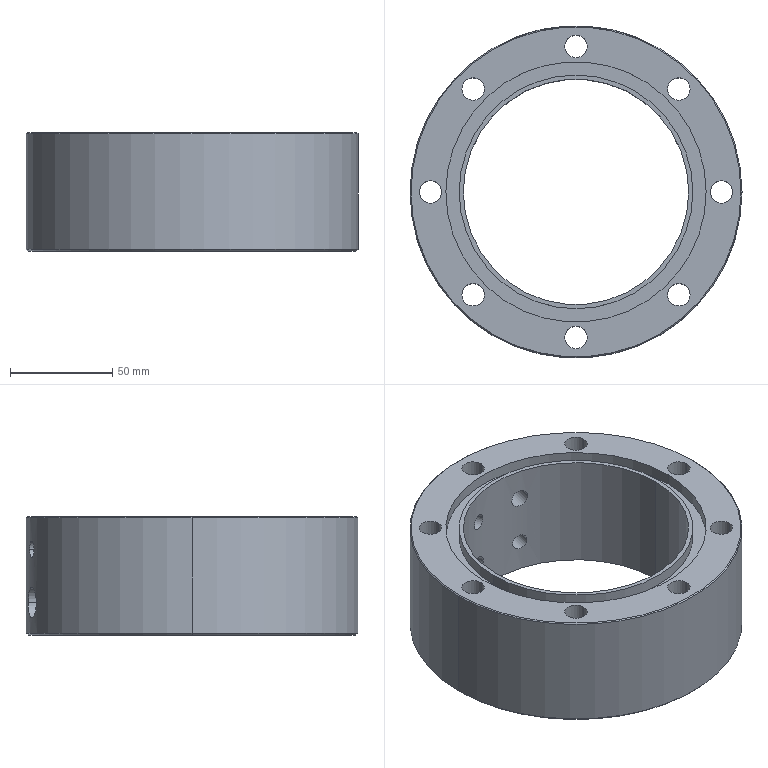Part | SolidWorks | features HoleWzd 5, 3DProfileFeature 4, Chamfer 2, ICE 2, CirPattern 1, Extrusion 1, MirrorPattern 1 | 1 solid | 52 faces | box 162 x 162 x 58 mm | volume 564661 mm3 | cylinder 40 | plane 8 | cone 4 | commonest cylinder face diameters 11 x16 8 x4 9 x4 15 x4 114 x4 127 x4